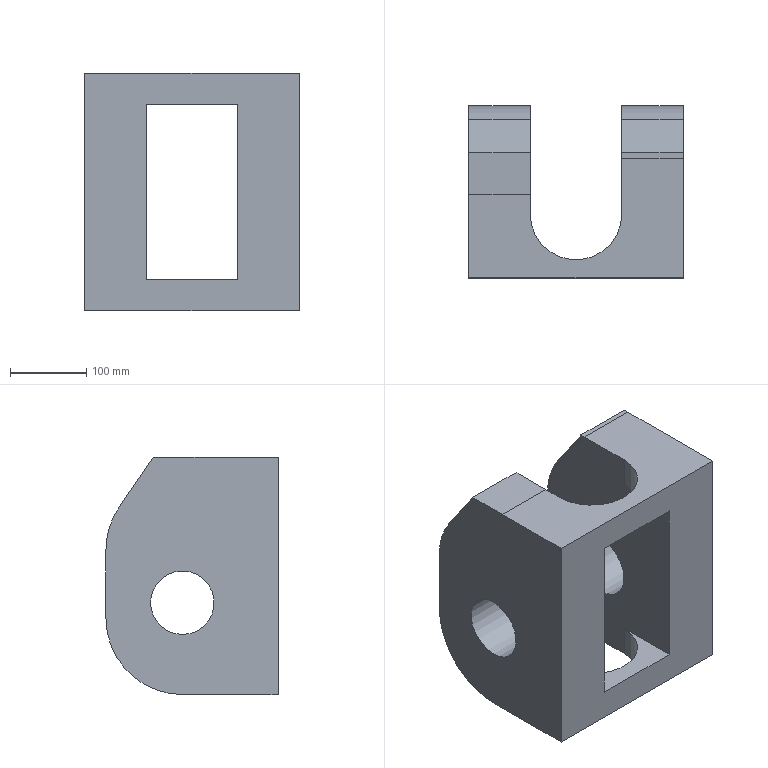Part | NX | features solid 2 | 1 solid | 25 faces | box 280 x 225 x 310 mm | volume 9841287 mm3 | plane 17 | cylinder 8 | commonest cylinder face diameters 200 x4 83 x2 120 x2
STEP:
#1=CARTESIAN_POINT('',(1335.,590.,10.));
#2=VERTEX_POINT('',#1);
#3=CARTESIAN_POINT('',(1215.,590.,10.));
#4=VERTEX_POINT('',#3);
#5=CARTESIAN_POINT('',(1495.,590.,10.));
#6=DIRECTION('',(-1.,0.,0.));
#7=VECTOR('',#6,1000.);
#8=LINE('',#5,#7);
#9=EDGE_CURVE('',#2,#4,#8,.T.);
#10=ORIENTED_EDGE('',*,*,#9,.T.);
#11=CARTESIAN_POINT('',(1215.,590.,240.));
#12=VERTEX_POINT('',#11);
#13=CARTESIAN_POINT('',(1215.,590.,-30.));
#14=DIRECTION('',(0.,0.,1.));
#15=VECTOR('',#14,1000.);
#16=LINE('',#13,#15);
#17=EDGE_CURVE('',#4,#12,#16,.T.);
#18=ORIENTED_EDGE('',*,*,#17,.T.);
#19=CARTESIAN_POINT('',(1335.,590.,240.));
#20=VERTEX_POINT('',#19);
#21=CARTESIAN_POINT('',(1440.,590.,240.));
#22=DIRECTION('',(-1.,0.,0.));
#23=VECTOR('',#22,1000.);
#24=LINE('',#21,#23);
#25=EDGE_CURVE('',#20,#12,#24,.T.);
#26=ORIENTED_EDGE('',*,*,#25,.F.);
#27=CARTESIAN_POINT('',(1335.,590.,-30.));
#28=DIRECTION('',(0.,0.,1.));
#29=VECTOR('',#28,1000.);
#30=LINE('',#27,#29);
#31=EDGE_CURVE('',#2,#20,#30,.T.);
#32=ORIENTED_EDGE('',*,*,#31,.F.);
#33=EDGE_LOOP('',(#10,#18,#26,#32));
#34=FACE_BOUND('',#33,.T.);
#35=CARTESIAN_POINT('',(1415.,590.,-30.));
#36=VERTEX_POINT('',#35);
#37=CARTESIAN_POINT('',(1415.,590.,280.));
#38=VERTEX_POINT('',#37);
#39=CARTESIAN_POINT('',(1415.,590.,-30.));
#40=DIRECTION('',(0.,0.,1.));
#41=VECTOR('',#40,1000.);
#42=LINE('',#39,#41);
#43=EDGE_CURVE('',#36,#38,#42,.T.);
#44=ORIENTED_EDGE('',*,*,#43,.T.);
#45=CARTESIAN_POINT('',(1135.,590.,280.));
#46=VERTEX_POINT('',#45);
#47=CARTESIAN_POINT('',(1405.,590.,280.));
#48=DIRECTION('',(-1.,0.,0.));
#49=VECTOR('',#48,1000.);
#50=LINE('',#47,#49);
#51=EDGE_CURVE('',#38,#46,#50,.T.);
#52=ORIENTED_EDGE('',*,*,#51,.T.);
#53=CARTESIAN_POINT('',(1135.,590.,-30.));
#54=VERTEX_POINT('',#53);
#55=CARTESIAN_POINT('',(1135.,590.,0.));
#56=DIRECTION('',(0.,0.,1.));
#57=VECTOR('',#56,1000.);
#58=LINE('',#55,#57);
#59=EDGE_CURVE('',#46,#54,#58,.F.);
#60=ORIENTED_EDGE('',*,*,#59,.T.);
#61=CARTESIAN_POINT('',(1135.,590.,-30.));
#62=DIRECTION('',(-1.,0.,0.));
#63=VECTOR('',#62,1000.);
#64=LINE('',#61,#63);
#65=EDGE_CURVE('',#36,#54,#64,.T.);
#66=ORIENTED_EDGE('',*,*,#65,.F.);
#67=EDGE_LOOP('',(#44,#52,#60,#66));
#68=FACE_BOUND('',#67,.T.);
#69=CARTESIAN_POINT('',(1135.,590.,0.));
#70=DIRECTION('',(0.,1.,0.));
#71=DIRECTION('',(0.,0.,-1.));
#72=AXIS2_PLACEMENT_3D('',#69,#70,#71);
#73=PLANE('',#72);
#74=ADVANCED_FACE('',(#34,#68),#73,.F.);
#75=ORIENTED_EDGE('',*,*,#51,.F.);
#76=CARTESIAN_POINT('',(1415.,746.5,280.));
#77=VERTEX_POINT('',#76);
#78=CARTESIAN_POINT('',(1415.,581.625,280.));
#79=DIRECTION('',(0.,-1.,0.));
#80=VECTOR('',#79,1000.);
#81=LINE('',#78,#80);
#82=EDGE_CURVE('',#38,#77,#81,.F.);
#83=ORIENTED_EDGE('',*,*,#82,.T.);
#84=CARTESIAN_POINT('',(1335.,746.5,280.));
#85=VERTEX_POINT('',#84);
#86=CARTESIAN_POINT('',(1405.,746.5,280.));
#87=DIRECTION('',(1.,0.,0.));
#88=VECTOR('',#87,1000.);
#89=LINE('',#86,#88);
#90=EDGE_CURVE('',#77,#85,#89,.F.);
#91=ORIENTED_EDGE('',*,*,#90,.T.);
#92=CARTESIAN_POINT('',(1335.,673.5,280.));
#93=VERTEX_POINT('',#92);
#94=CARTESIAN_POINT('',(1335.,590.,280.));
#95=DIRECTION('',(0.,-1.,0.));
#96=VECTOR('',#95,1000.);
#97=LINE('',#94,#96);
#98=EDGE_CURVE('',#93,#85,#97,.F.);
#99=ORIENTED_EDGE('',*,*,#98,.F.);
#100=CARTESIAN_POINT('',(1215.,673.5,280.));
#101=VERTEX_POINT('',#100);
#102=CARTESIAN_POINT('',(1275.,673.5,280.));
#103=DIRECTION('',(0.,0.,1.));
#104=DIRECTION('',(1.,0.,0.));
#105=AXIS2_PLACEMENT_3D('',#102,#103,#104);
#106=CIRCLE('',#105,60.);
#107=EDGE_CURVE('',#101,#93,#106,.T.);
#108=ORIENTED_EDGE('',*,*,#107,.F.);
#109=CARTESIAN_POINT('',(1215.,698.55,280.));
#110=VERTEX_POINT('',#109);
#111=CARTESIAN_POINT('',(1215.,581.625,280.));
#112=DIRECTION('',(0.,1.,0.));
#113=VECTOR('',#112,1000.);
#114=LINE('',#111,#113);
#115=EDGE_CURVE('',#110,#101,#114,.F.);
#116=ORIENTED_EDGE('',*,*,#115,.F.);
#117=CARTESIAN_POINT('',(1135.,698.55,280.));
#118=VERTEX_POINT('',#117);
#119=CARTESIAN_POINT('',(1405.,698.55,280.));
#120=DIRECTION('',(1.,0.,0.));
#121=VECTOR('',#120,1000.);
#122=LINE('',#119,#121);
#123=EDGE_CURVE('',#110,#118,#122,.F.);
#124=ORIENTED_EDGE('',*,*,#123,.T.);
#125=CARTESIAN_POINT('',(1135.,581.625,280.));
#126=DIRECTION('',(0.,-1.,0.));
#127=VECTOR('',#126,1000.);
#128=LINE('',#125,#127);
#129=EDGE_CURVE('',#46,#118,#128,.F.);
#130=ORIENTED_EDGE('',*,*,#129,.F.);
#131=EDGE_LOOP('',(#75,#83,#91,#99,#108,#116,#124,#130));
#132=FACE_BOUND('',#131,.T.);
#133=CARTESIAN_POINT('',(1405.,581.625,280.));
#134=DIRECTION('',(0.,0.,-1.));
#135=DIRECTION('',(-1.,0.,0.));
#136=AXIS2_PLACEMENT_3D('',#133,#134,#135);
#137=PLANE('',#136);
#138=ADVANCED_FACE('',(#132),#137,.F.);
#139=CARTESIAN_POINT('',(1135.,715.,-30.));
#140=VERTEX_POINT('',#139);
#141=CARTESIAN_POINT('',(1135.,530.,-30.));
#142=DIRECTION('',(0.,1.,0.));
#143=VECTOR('',#142,1000.);
#144=LINE('',#141,#143);
#145=EDGE_CURVE('',#140,#54,#144,.F.);
#146=ORIENTED_EDGE('',*,*,#145,.T.);
#147=ORIENTED_EDGE('',*,*,#59,.F.);
#148=ORIENTED_EDGE('',*,*,#129,.T.);
#149=CARTESIAN_POINT('',(1135.,753.35,280.));
#150=VERTEX_POINT('',#149);
#151=CARTESIAN_POINT('',(1135.,530.,280.));
#152=DIRECTION('',(0.,1.,0.));
#153=VECTOR('',#152,1000.);
#154=LINE('',#151,#153);
#155=EDGE_CURVE('',#150,#118,#154,.F.);
#156=ORIENTED_EDGE('',*,*,#155,.F.);
#157=CARTESIAN_POINT('',(1135.,797.5,215.547));
#158=VERTEX_POINT('',#157);
#159=CARTESIAN_POINT('',(1135.,826.551,173.137));
#160=DIRECTION('',(0.,-0.5651,0.825));
#161=VECTOR('',#160,1000.);
#162=LINE('',#159,#161);
#163=EDGE_CURVE('',#158,#150,#162,.T.);
#164=ORIENTED_EDGE('',*,*,#163,.F.);
#165=CARTESIAN_POINT('',(1135.,815.,159.034));
#166=VERTEX_POINT('',#165);
#167=CARTESIAN_POINT('',(1135.,715.,159.034));
#168=DIRECTION('',(-1.,0.,0.));
#169=DIRECTION('',(0.,0.,1.));
#170=AXIS2_PLACEMENT_3D('',#167,#168,#169);
#171=CIRCLE('',#170,100.);
#172=EDGE_CURVE('',#166,#158,#171,.F.);
#173=ORIENTED_EDGE('',*,*,#172,.F.);
#174=CARTESIAN_POINT('',(1135.,815.,70.));
#175=VERTEX_POINT('',#174);
#176=CARTESIAN_POINT('',(1135.,815.,-30.));
#177=DIRECTION('',(0.,0.,-1.));
#178=VECTOR('',#177,1000.);
#179=LINE('',#176,#178);
#180=EDGE_CURVE('',#175,#166,#179,.F.);
#181=ORIENTED_EDGE('',*,*,#180,.F.);
#182=CARTESIAN_POINT('',(1135.,715.,70.));
#183=DIRECTION('',(-1.,0.,0.));
#184=DIRECTION('',(0.,0.,1.));
#185=AXIS2_PLACEMENT_3D('',#182,#183,#184);
#186=CIRCLE('',#185,100.);
#187=EDGE_CURVE('',#140,#175,#186,.F.);
#188=ORIENTED_EDGE('',*,*,#187,.F.);
#189=EDGE_LOOP('',(#146,#147,#148,#156,#164,#173,#181,#188));
#190=FACE_BOUND('',#189,.T.);
#191=CARTESIAN_POINT('',(1135.,715.,48.5));
#192=VERTEX_POINT('',#191);
#193=CARTESIAN_POINT('',(1135.,715.,90.));
#194=DIRECTION('',(1.,0.,0.));
#195=DIRECTION('',(0.,0.,-1.));
#196=AXIS2_PLACEMENT_3D('',#193,#194,#195);
#197=CIRCLE('',#196,41.5);
#198=EDGE_CURVE('',#192,#192,#197,.T.);
#199=ORIENTED_EDGE('',*,*,#198,.T.);
#200=EDGE_LOOP('',(#199));
#201=FACE_BOUND('',#200,.T.);
#202=CARTESIAN_POINT('',(1135.,530.,-30.));
#203=DIRECTION('',(1.,0.,0.));
#204=DIRECTION('',(0.,0.,-1.));
#205=AXIS2_PLACEMENT_3D('',#202,#203,#204);
#206=PLANE('',#205);
#207=ADVANCED_FACE('',(#190,#201),#206,.F.);
#208=CARTESIAN_POINT('',(1335.,715.,48.5));
#209=VERTEX_POINT('',#208);
#210=CARTESIAN_POINT('',(1335.,715.,90.));
#211=DIRECTION('',(1.,0.,0.));
#212=DIRECTION('',(0.,0.,-1.));
#213=AXIS2_PLACEMENT_3D('',#210,#211,#212);
#214=CIRCLE('',#213,41.5);
#215=EDGE_CURVE('',#209,#209,#214,.T.);
#216=ORIENTED_EDGE('',*,*,#215,.T.);
#217=EDGE_LOOP('',(#216));
#218=FACE_BOUND('',#217,.T.);
#219=CARTESIAN_POINT('',(1335.,749.714,280.));
#220=VERTEX_POINT('',#219);
#221=CARTESIAN_POINT('',(1335.,590.,280.));
#222=DIRECTION('',(0.,1.,0.));
#223=VECTOR('',#222,1000.);
#224=LINE('',#221,#223);
#225=EDGE_CURVE('',#220,#85,#224,.F.);
#226=ORIENTED_EDGE('',*,*,#225,.F.);
#227=CARTESIAN_POINT('',(1335.,795.025,213.852));
#228=VERTEX_POINT('',#227);
#229=CARTESIAN_POINT('',(1335.,795.025,213.852));
#230=DIRECTION('',(0.,-0.5651,0.825));
#231=VECTOR('',#230,1000.);
#232=LINE('',#229,#231);
#233=EDGE_CURVE('',#220,#228,#232,.F.);
#234=ORIENTED_EDGE('',*,*,#233,.T.);
#235=CARTESIAN_POINT('',(1335.,812.,159.034));
#236=VERTEX_POINT('',#235);
#237=CARTESIAN_POINT('',(1335.,715.,159.034));
#238=DIRECTION('',(1.,0.,0.));
#239=DIRECTION('',(0.,0.,-1.));
#240=AXIS2_PLACEMENT_3D('',#237,#238,#239);
#241=CIRCLE('',#240,97.);
#242=EDGE_CURVE('',#228,#236,#241,.F.);
#243=ORIENTED_EDGE('',*,*,#242,.T.);
#244=CARTESIAN_POINT('',(1335.,812.,70.));
#245=VERTEX_POINT('',#244);
#246=CARTESIAN_POINT('',(1335.,812.,70.));
#247=DIRECTION('',(0.,0.,1.));
#248=VECTOR('',#247,1000.);
#249=LINE('',#246,#248);
#250=EDGE_CURVE('',#236,#245,#249,.F.);
#251=ORIENTED_EDGE('',*,*,#250,.T.);
#252=CARTESIAN_POINT('',(1335.,715.,-27.));
#253=VERTEX_POINT('',#252);
#254=CARTESIAN_POINT('',(1335.,715.,70.));
#255=DIRECTION('',(1.,0.,0.));
#256=DIRECTION('',(0.,0.,-1.));
#257=AXIS2_PLACEMENT_3D('',#254,#255,#256);
#258=CIRCLE('',#257,97.);
#259=EDGE_CURVE('',#245,#253,#258,.F.);
#260=ORIENTED_EDGE('',*,*,#259,.T.);
#261=CARTESIAN_POINT('',(1335.,673.5,-27.));
#262=VERTEX_POINT('',#261);
#263=CARTESIAN_POINT('',(1335.,673.5,-27.));
#264=DIRECTION('',(0.,1.,0.));
#265=VECTOR('',#264,1000.);
#266=LINE('',#263,#265);
#267=EDGE_CURVE('',#253,#262,#266,.F.);
#268=ORIENTED_EDGE('',*,*,#267,.T.);
#269=CARTESIAN_POINT('',(1335.,673.5,10.));
#270=VERTEX_POINT('',#269);
#271=CARTESIAN_POINT('',(1335.,673.5,-30.));
#272=DIRECTION('',(0.,0.,1.));
#273=VECTOR('',#272,1000.);
#274=LINE('',#271,#273);
#275=EDGE_CURVE('',#262,#270,#274,.T.);
#276=ORIENTED_EDGE('',*,*,#275,.T.);
#277=CARTESIAN_POINT('',(1335.,590.,10.));
#278=DIRECTION('',(0.,1.,0.));
#279=VECTOR('',#278,1000.);
#280=LINE('',#277,#279);
#281=EDGE_CURVE('',#2,#270,#280,.T.);
#282=ORIENTED_EDGE('',*,*,#281,.F.);
#283=ORIENTED_EDGE('',*,*,#31,.T.);
#284=CARTESIAN_POINT('',(1335.,673.5,240.));
#285=VERTEX_POINT('',#284);
#286=CARTESIAN_POINT('',(1335.,690.,240.));
#287=DIRECTION('',(0.,1.,0.));
#288=VECTOR('',#287,1000.);
#289=LINE('',#286,#288);
#290=EDGE_CURVE('',#20,#285,#289,.T.);
#291=ORIENTED_EDGE('',*,*,#290,.T.);
#292=CARTESIAN_POINT('',(1335.,673.5,330.));
#293=DIRECTION('',(0.,0.,-1.));
#294=VECTOR('',#293,1000.);
#295=LINE('',#292,#294);
#296=EDGE_CURVE('',#93,#285,#295,.T.);
#297=ORIENTED_EDGE('',*,*,#296,.F.);
#298=ORIENTED_EDGE('',*,*,#98,.T.);
#299=EDGE_LOOP('',(#226,#234,#243,#251,#260,#268,#276,#282,#283,#291,#297,#298));
#300=FACE_BOUND('',#299,.T.);
#301=CARTESIAN_POINT('',(1335.,590.,-30.));
#302=DIRECTION('',(1.,0.,0.));
#303=DIRECTION('',(0.,0.,-1.));
#304=AXIS2_PLACEMENT_3D('',#301,#302,#303);
#305=PLANE('',#304);
#306=ADVANCED_FACE('',(#218,#300),#305,.F.);
#307=CARTESIAN_POINT('',(1215.,715.,48.5));
#308=VERTEX_POINT('',#307);
#309=CARTESIAN_POINT('',(1215.,715.,90.));
#310=DIRECTION('',(1.,0.,0.));
#311=DIRECTION('',(0.,0.,-1.));
#312=AXIS2_PLACEMENT_3D('',#309,#310,#311);
#313=CIRCLE('',#312,41.5);
#314=EDGE_CURVE('',#308,#308,#313,.T.);
#315=ORIENTED_EDGE('',*,*,#314,.F.);
#316=EDGE_LOOP('',(#315));
#317=FACE_BOUND('',#316,.T.);
#318=CARTESIAN_POINT('',(1215.,795.025,213.852));
#319=VERTEX_POINT('',#318);
#320=CARTESIAN_POINT('',(1215.,749.714,280.));
#321=VERTEX_POINT('',#320);
#322=CARTESIAN_POINT('',(1215.,843.238,143.468));
#323=DIRECTION('',(0.,0.5651,-0.825));
#324=VECTOR('',#323,1000.);
#325=LINE('',#322,#324);
#326=EDGE_CURVE('',#319,#321,#325,.F.);
#327=ORIENTED_EDGE('',*,*,#326,.T.);
#328=CARTESIAN_POINT('',(1215.,590.,280.));
#329=DIRECTION('',(0.,1.,0.));
#330=VECTOR('',#329,1000.);
#331=LINE('',#328,#330);
#332=EDGE_CURVE('',#321,#110,#331,.F.);
#333=ORIENTED_EDGE('',*,*,#332,.T.);
#334=ORIENTED_EDGE('',*,*,#115,.T.);
#335=CARTESIAN_POINT('',(1215.,673.5,240.));
#336=VERTEX_POINT('',#335);
#337=CARTESIAN_POINT('',(1215.,673.5,330.));
#338=DIRECTION('',(0.,0.,-1.));
#339=VECTOR('',#338,1000.);
#340=LINE('',#337,#339);
#341=EDGE_CURVE('',#101,#336,#340,.T.);
#342=ORIENTED_EDGE('',*,*,#341,.T.);
#343=CARTESIAN_POINT('',(1215.,690.,240.));
#344=DIRECTION('',(0.,1.,0.));
#345=VECTOR('',#344,1000.);
#346=LINE('',#343,#345);
#347=EDGE_CURVE('',#12,#336,#346,.T.);
#348=ORIENTED_EDGE('',*,*,#347,.F.);
#349=ORIENTED_EDGE('',*,*,#17,.F.);
#350=CARTESIAN_POINT('',(1215.,673.5,10.));
#351=VERTEX_POINT('',#350);
#352=CARTESIAN_POINT('',(1215.,590.,10.));
#353=DIRECTION('',(0.,1.,0.));
#354=VECTOR('',#353,1000.);
#355=LINE('',#352,#354);
#356=EDGE_CURVE('',#4,#351,#355,.T.);
#357=ORIENTED_EDGE('',*,*,#356,.T.);
#358=CARTESIAN_POINT('',(1215.,673.5,-27.));
#359=VERTEX_POINT('',#358);
#360=CARTESIAN_POINT('',(1215.,673.5,-30.));
#361=DIRECTION('',(0.,0.,1.));
#362=VECTOR('',#361,1000.);
#363=LINE('',#360,#362);
#364=EDGE_CURVE('',#359,#351,#363,.T.);
#365=ORIENTED_EDGE('',*,*,#364,.F.);
#366=CARTESIAN_POINT('',(1215.,715.,-27.));
#367=VERTEX_POINT('',#366);
#368=CARTESIAN_POINT('',(1215.,590.,-27.));
#369=DIRECTION('',(0.,1.,0.));
#370=VECTOR('',#369,1000.);
#371=LINE('',#368,#370);
#372=EDGE_CURVE('',#359,#367,#371,.T.);
#373=ORIENTED_EDGE('',*,*,#372,.T.);
#374=CARTESIAN_POINT('',(1215.,812.,70.));
#375=VERTEX_POINT('',#374);
#376=CARTESIAN_POINT('',(1215.,715.,70.));
#377=DIRECTION('',(1.,0.,0.));
#378=DIRECTION('',(0.,0.,-1.));
#379=AXIS2_PLACEMENT_3D('',#376,#377,#378);
#380=CIRCLE('',#379,97.);
#381=EDGE_CURVE('',#367,#375,#380,.T.);
#382=ORIENTED_EDGE('',*,*,#381,.T.);
#383=CARTESIAN_POINT('',(1215.,812.,159.034));
#384=VERTEX_POINT('',#383);
#385=CARTESIAN_POINT('',(1215.,812.,-30.));
#386=DIRECTION('',(0.,0.,1.));
#387=VECTOR('',#386,1000.);
#388=LINE('',#385,#387);
#389=EDGE_CURVE('',#375,#384,#388,.T.);
#390=ORIENTED_EDGE('',*,*,#389,.T.);
#391=CARTESIAN_POINT('',(1215.,715.,159.034));
#392=DIRECTION('',(1.,0.,0.));
#393=DIRECTION('',(0.,0.,-1.));
#394=AXIS2_PLACEMENT_3D('',#391,#392,#393);
#395=CIRCLE('',#394,97.);
#396=EDGE_CURVE('',#384,#319,#395,.T.);
#397=ORIENTED_EDGE('',*,*,#396,.T.);
#398=EDGE_LOOP('',(#327,#333,#334,#342,#348,#349,#357,#365,#373,#382,#390,#397));
#399=FACE_BOUND('',#398,.T.);
#400=CARTESIAN_POINT('',(1215.,590.,-30.));
#401=DIRECTION('',(1.,0.,0.));
#402=DIRECTION('',(0.,0.,-1.));
#403=AXIS2_PLACEMENT_3D('',#400,#401,#402);
#404=PLANE('',#403);
#405=ADVANCED_FACE('',(#317,#399),#404,.T.);
#406=ORIENTED_EDGE('',*,*,#82,.F.);
#407=ORIENTED_EDGE('',*,*,#43,.F.);
#408=CARTESIAN_POINT('',(1415.,715.,-30.));
#409=VERTEX_POINT('',#408);
#410=CARTESIAN_POINT('',(1415.,530.,-30.));
#411=DIRECTION('',(0.,1.,0.));
#412=VECTOR('',#411,1000.);
#413=LINE('',#410,#412);
#414=EDGE_CURVE('',#36,#409,#413,.T.);
#415=ORIENTED_EDGE('',*,*,#414,.T.);
#416=CARTESIAN_POINT('',(1415.,815.,70.));
#417=VERTEX_POINT('',#416);
#418=CARTESIAN_POINT('',(1415.,715.,70.));
#419=DIRECTION('',(-1.,0.,0.));
#420=DIRECTION('',(0.,0.,1.));
#421=AXIS2_PLACEMENT_3D('',#418,#419,#420);
#422=CIRCLE('',#421,100.);
#423=EDGE_CURVE('',#417,#409,#422,.T.);
#424=ORIENTED_EDGE('',*,*,#423,.F.);
#425=CARTESIAN_POINT('',(1415.,815.,159.034));
#426=VERTEX_POINT('',#425);
#427=CARTESIAN_POINT('',(1415.,815.,-30.));
#428=DIRECTION('',(0.,0.,1.));
#429=VECTOR('',#428,1000.);
#430=LINE('',#427,#429);
#431=EDGE_CURVE('',#426,#417,#430,.F.);
#432=ORIENTED_EDGE('',*,*,#431,.F.);
#433=CARTESIAN_POINT('',(1415.,797.5,215.547));
#434=VERTEX_POINT('',#433);
#435=CARTESIAN_POINT('',(1415.,715.,159.034));
#436=DIRECTION('',(-1.,0.,0.));
#437=DIRECTION('',(0.,0.,1.));
#438=AXIS2_PLACEMENT_3D('',#435,#436,#437);
#439=CIRCLE('',#438,100.);
#440=EDGE_CURVE('',#434,#426,#439,.T.);
#441=ORIENTED_EDGE('',*,*,#440,.F.);
#442=CARTESIAN_POINT('',(1415.,753.35,280.));
#443=VERTEX_POINT('',#442);
#444=CARTESIAN_POINT('',(1415.,845.713,145.163));
#445=DIRECTION('',(0.,-0.5651,0.825));
#446=VECTOR('',#445,1000.);
#447=LINE('',#444,#446);
#448=EDGE_CURVE('',#443,#434,#447,.F.);
#449=ORIENTED_EDGE('',*,*,#448,.F.);
#450=CARTESIAN_POINT('',(1415.,530.,280.));
#451=DIRECTION('',(0.,1.,0.));
#452=VECTOR('',#451,1000.);
#453=LINE('',#450,#452);
#454=EDGE_CURVE('',#443,#77,#453,.F.);
#455=ORIENTED_EDGE('',*,*,#454,.T.);
#456=EDGE_LOOP('',(#406,#407,#415,#424,#432,#441,#449,#455));
#457=FACE_BOUND('',#456,.T.);
#458=CARTESIAN_POINT('',(1415.,715.,131.5));
#459=VERTEX_POINT('',#458);
#460=CARTESIAN_POINT('',(1415.,715.,90.));
#461=DIRECTION('',(-1.,0.,0.));
#462=DIRECTION('',(0.,0.,1.));
#463=AXIS2_PLACEMENT_3D('',#460,#461,#462);
#464=CIRCLE('',#463,41.5);
#465=EDGE_CURVE('',#459,#459,#464,.T.);
#466=ORIENTED_EDGE('',*,*,#465,.T.);
#467=EDGE_LOOP('',(#466));
#468=FACE_BOUND('',#467,.T.);
#469=CARTESIAN_POINT('',(1415.,530.,-30.));
#470=DIRECTION('',(1.,0.,0.));
#471=DIRECTION('',(0.,0.,-1.));
#472=AXIS2_PLACEMENT_3D('',#469,#470,#471);
#473=PLANE('',#472);
#474=ADVANCED_FACE('',(#457,#468),#473,.T.);
#475=ORIENTED_EDGE('',*,*,#107,.T.);
#476=ORIENTED_EDGE('',*,*,#296,.T.);
#477=CARTESIAN_POINT('',(1275.,673.5,240.));
#478=DIRECTION('',(0.,0.,1.));
#479=DIRECTION('',(1.,0.,0.));
#480=AXIS2_PLACEMENT_3D('',#477,#478,#479);
#481=CIRCLE('',#480,60.);
#482=EDGE_CURVE('',#285,#336,#481,.F.);
#483=ORIENTED_EDGE('',*,*,#482,.T.);
#484=ORIENTED_EDGE('',*,*,#341,.F.);
#485=EDGE_LOOP('',(#475,#476,#483,#484));
#486=FACE_BOUND('',#485,.T.);
#487=CARTESIAN_POINT('',(1275.,673.5,330.));
#488=DIRECTION('',(0.,0.,-1.));
#489=DIRECTION('',(-1.,0.,0.));
#490=AXIS2_PLACEMENT_3D('',#487,#488,#489);
#491=CYLINDRICAL_SURFACE('',#490,60.);
#492=ADVANCED_FACE('',(#486),#491,.F.);
#493=ORIENTED_EDGE('',*,*,#233,.F.);
#494=CARTESIAN_POINT('',(1335.,753.35,280.));
#495=VERTEX_POINT('',#494);
#496=CARTESIAN_POINT('',(1335.,581.625,280.));
#497=DIRECTION('',(0.,-1.,0.));
#498=VECTOR('',#497,1000.);
#499=LINE('',#496,#498);
#500=EDGE_CURVE('',#495,#220,#499,.T.);
#501=ORIENTED_EDGE('',*,*,#500,.F.);
#502=CARTESIAN_POINT('',(1335.,797.5,215.547));
#503=VERTEX_POINT('',#502);
#504=CARTESIAN_POINT('',(1335.,845.713,145.163));
#505=DIRECTION('',(0.,-0.5651,0.825));
#506=VECTOR('',#505,1000.);
#507=LINE('',#504,#506);
#508=EDGE_CURVE('',#503,#495,#507,.T.);
#509=ORIENTED_EDGE('',*,*,#508,.F.);
#510=CARTESIAN_POINT('',(1335.,815.,159.034));
#511=VERTEX_POINT('',#510);
#512=CARTESIAN_POINT('',(1335.,715.,159.034));
#513=DIRECTION('',(-1.,0.,0.));
#514=DIRECTION('',(0.,0.,1.));
#515=AXIS2_PLACEMENT_3D('',#512,#513,#514);
#516=CIRCLE('',#515,100.);
#517=EDGE_CURVE('',#511,#503,#516,.F.);
#518=ORIENTED_EDGE('',*,*,#517,.F.);
#519=CARTESIAN_POINT('',(1335.,815.,70.));
#520=VERTEX_POINT('',#519);
#521=CARTESIAN_POINT('',(1335.,815.,-30.));
#522=DIRECTION('',(0.,0.,-1.));
#523=VECTOR('',#522,1000.);
#524=LINE('',#521,#523);
#525=EDGE_CURVE('',#520,#511,#524,.F.);
#526=ORIENTED_EDGE('',*,*,#525,.F.);
#527=CARTESIAN_POINT('',(1335.,715.,-30.));
#528=VERTEX_POINT('',#527);
#529=CARTESIAN_POINT('',(1335.,715.,70.));
#530=DIRECTION('',(-1.,0.,0.));
#531=DIRECTION('',(0.,0.,1.));
#532=AXIS2_PLACEMENT_3D('',#529,#530,#531);
#533=CIRCLE('',#532,100.);
#534=EDGE_CURVE('',#528,#520,#533,.F.);
#535=ORIENTED_EDGE('',*,*,#534,.F.);
#536=CARTESIAN_POINT('',(1335.,673.5,-30.));
#537=VERTEX_POINT('',#536);
#538=CARTESIAN_POINT('',(1335.,590.,-30.));
#539=DIRECTION('',(0.,-1.,0.));
#540=VECTOR('',#539,1000.);
#541=LINE('',#538,#540);
#542=EDGE_CURVE('',#537,#528,#541,.F.);
#543=ORIENTED_EDGE('',*,*,#542,.F.);
#544=CARTESIAN_POINT('',(1335.,673.5,-30.));
#545=DIRECTION('',(0.,0.,1.));
#546=VECTOR('',#545,1000.);
#547=LINE('',#544,#546);
#548=EDGE_CURVE('',#262,#537,#547,.F.);
#549=ORIENTED_EDGE('',*,*,#548,.F.);
#550=ORIENTED_EDGE('',*,*,#267,.F.);
#551=ORIENTED_EDGE('',*,*,#259,.F.);
#552=ORIENTED_EDGE('',*,*,#250,.F.);
#553=ORIENTED_EDGE('',*,*,#242,.F.);
#554=EDGE_LOOP('',(#493,#501,#509,#518,#526,#535,#543,#549,#550,#551,#552,#553));
#555=FACE_BOUND('',#554,.T.);
#556=CARTESIAN_POINT('',(1335.,590.,-30.));
#557=DIRECTION('',(1.,0.,0.));
#558=DIRECTION('',(0.,0.,-1.));
#559=AXIS2_PLACEMENT_3D('',#556,#557,#558);
#560=PLANE('',#559);
#561=ADVANCED_FACE('',(#555),#560,.F.);
#562=ORIENTED_EDGE('',*,*,#65,.T.);
#563=ORIENTED_EDGE('',*,*,#145,.F.);
#564=CARTESIAN_POINT('',(1215.,715.,-30.));
#565=VERTEX_POINT('',#564);
#566=CARTESIAN_POINT('',(1405.,715.,-30.));
#567=DIRECTION('',(-1.,0.,0.));
#568=VECTOR('',#567,1000.);
#569=LINE('',#566,#568);
#570=EDGE_CURVE('',#140,#565,#569,.F.);
#571=ORIENTED_EDGE('',*,*,#570,.T.);
#572=CARTESIAN_POINT('',(1215.,673.5,-30.));
#573=VERTEX_POINT('',#572);
#574=CARTESIAN_POINT('',(1215.,590.,-30.));
#575=DIRECTION('',(0.,-1.,0.));
#576=VECTOR('',#575,1000.);
#577=LINE('',#574,#576);
#578=EDGE_CURVE('',#565,#573,#577,.T.);
#579=ORIENTED_EDGE('',*,*,#578,.T.);
#580=CARTESIAN_POINT('',(1275.,673.5,-30.));
#581=DIRECTION('',(0.,0.,1.));
#582=DIRECTION('',(1.,0.,0.));
#583=AXIS2_PLACEMENT_3D('',#580,#581,#582);
#584=CIRCLE('',#583,60.);
#585=EDGE_CURVE('',#573,#537,#584,.T.);
#586=ORIENTED_EDGE('',*,*,#585,.T.);
#587=ORIENTED_EDGE('',*,*,#542,.T.);
#588=CARTESIAN_POINT('',(1405.,715.,-30.));
#589=DIRECTION('',(-1.,0.,0.));
#590=VECTOR('',#589,1000.);
#591=LINE('',#588,#590);
#592=EDGE_CURVE('',#528,#409,#591,.F.);
#593=ORIENTED_EDGE('',*,*,#592,.T.);
#594=ORIENTED_EDGE('',*,*,#414,.F.);
#595=EDGE_LOOP('',(#562,#563,#571,#579,#586,#587,#593,#594));
#596=FACE_BOUND('',#595,.T.);
#597=CARTESIAN_POINT('',(1405.,581.625,-30.));
#598=DIRECTION('',(0.,0.,-1.));
#599=DIRECTION('',(-1.,0.,0.));
#600=AXIS2_PLACEMENT_3D('',#597,#598,#599);
#601=PLANE('',#600);
#602=ADVANCED_FACE('',(#596),#601,.T.);
#603=CARTESIAN_POINT('',(1415.,815.,70.));
#604=DIRECTION('',(-1.,0.,0.));
#605=VECTOR('',#604,1000.);
#606=LINE('',#603,#605);
#607=EDGE_CURVE('',#417,#520,#606,.T.);
#608=ORIENTED_EDGE('',*,*,#607,.T.);
#609=ORIENTED_EDGE('',*,*,#525,.T.);
#610=CARTESIAN_POINT('',(1415.,815.,159.034));
#611=DIRECTION('',(-1.,0.,0.));
#612=VECTOR('',#611,1000.);
#613=LINE('',#610,#612);
#614=EDGE_CURVE('',#511,#426,#613,.F.);
#615=ORIENTED_EDGE('',*,*,#614,.T.);
#616=ORIENTED_EDGE('',*,*,#431,.T.);
#617=EDGE_LOOP('',(#608,#609,#615,#616));
#618=FACE_BOUND('',#617,.T.);
#619=CARTESIAN_POINT('',(1415.,815.,-30.));
#620=DIRECTION('',(0.,1.,0.));
#621=DIRECTION('',(0.,0.,-1.));
#622=AXIS2_PLACEMENT_3D('',#619,#620,#621);
#623=PLANE('',#622);
#624=ADVANCED_FACE('',(#618),#623,.T.);
#625=CARTESIAN_POINT('',(1215.,815.,70.));
#626=VERTEX_POINT('',#625);
#627=CARTESIAN_POINT('',(1215.,815.,70.));
#628=DIRECTION('',(-1.,0.,0.));
#629=VECTOR('',#628,1000.);
#630=LINE('',#627,#629);
#631=EDGE_CURVE('',#626,#175,#630,.T.);
#632=ORIENTED_EDGE('',*,*,#631,.T.);
#633=ORIENTED_EDGE('',*,*,#180,.T.);
#634=CARTESIAN_POINT('',(1215.,815.,159.034));
#635=VERTEX_POINT('',#634);
#636=CARTESIAN_POINT('',(1215.,815.,159.034));
#637=DIRECTION('',(-1.,0.,0.));
#638=VECTOR('',#637,1000.);
#639=LINE('',#636,#638);
#640=EDGE_CURVE('',#166,#635,#639,.F.);
#641=ORIENTED_EDGE('',*,*,#640,.T.);
#642=CARTESIAN_POINT('',(1215.,815.,-30.));
#643=DIRECTION('',(0.,0.,-1.));
#644=VECTOR('',#643,1000.);
#645=LINE('',#642,#644);
#646=EDGE_CURVE('',#635,#626,#645,.T.);
#647=ORIENTED_EDGE('',*,*,#646,.T.);
#648=EDGE_LOOP('',(#632,#633,#641,#647));
#649=FACE_BOUND('',#648,.T.);
#650=CARTESIAN_POINT('',(1215.,815.,-30.));
#651=DIRECTION('',(0.,1.,0.));
#652=DIRECTION('',(0.,0.,-1.));
#653=AXIS2_PLACEMENT_3D('',#650,#651,#652);
#654=PLANE('',#653);
#655=ADVANCED_FACE('',(#649),#654,.T.);
#656=ORIENTED_EDGE('',*,*,#364,.T.);
#657=CARTESIAN_POINT('',(1275.,673.5,10.));
#658=DIRECTION('',(0.,0.,-1.));
#659=DIRECTION('',(-1.,0.,0.));
#660=AXIS2_PLACEMENT_3D('',#657,#658,#659);
#661=CIRCLE('',#660,60.);
#662=EDGE_CURVE('',#351,#270,#661,.F.);
#663=ORIENTED_EDGE('',*,*,#662,.T.);
#664=ORIENTED_EDGE('',*,*,#275,.F.);
#665=ORIENTED_EDGE('',*,*,#548,.T.);
#666=ORIENTED_EDGE('',*,*,#585,.F.);
#667=CARTESIAN_POINT('',(1215.,673.5,-30.));
#668=DIRECTION('',(0.,0.,1.));
#669=VECTOR('',#668,1000.);
#670=LINE('',#667,#669);
#671=EDGE_CURVE('',#359,#573,#670,.F.);
#672=ORIENTED_EDGE('',*,*,#671,.F.);
#673=EDGE_LOOP('',(#656,#663,#664,#665,#666,#672));
#674=FACE_BOUND('',#673,.T.);
#675=CARTESIAN_POINT('',(1275.,673.5,-30.));
#676=DIRECTION('',(0.,0.,1.));
#677=DIRECTION('',(1.,0.,0.));
#678=AXIS2_PLACEMENT_3D('',#675,#676,#677);
#679=CYLINDRICAL_SURFACE('',#678,60.);
#680=ADVANCED_FACE('',(#674),#679,.F.);
#681=ORIENTED_EDGE('',*,*,#281,.T.);
#682=ORIENTED_EDGE('',*,*,#662,.F.);
#683=ORIENTED_EDGE('',*,*,#356,.F.);
#684=ORIENTED_EDGE('',*,*,#9,.F.);
#685=EDGE_LOOP('',(#681,#682,#683,#684));
#686=FACE_BOUND('',#685,.T.);
#687=CARTESIAN_POINT('',(1285.,659.625,10.));
#688=DIRECTION('',(0.,0.,1.));
#689=DIRECTION('',(1.,0.,0.));
#690=AXIS2_PLACEMENT_3D('',#687,#688,#689);
#691=PLANE('',#690);
#692=ADVANCED_FACE('',(#686),#691,.T.);
#693=ORIENTED_EDGE('',*,*,#570,.F.);
#694=ORIENTED_EDGE('',*,*,#187,.T.);
#695=ORIENTED_EDGE('',*,*,#631,.F.);
#696=CARTESIAN_POINT('',(1215.,715.,70.));
#697=DIRECTION('',(-1.,0.,0.));
#698=DIRECTION('',(0.,0.,1.));
#699=AXIS2_PLACEMENT_3D('',#696,#697,#698);
#700=CIRCLE('',#699,100.);
#701=EDGE_CURVE('',#626,#565,#700,.T.);
#702=ORIENTED_EDGE('',*,*,#701,.T.);
#703=EDGE_LOOP('',(#693,#694,#695,#702));
#704=FACE_BOUND('',#703,.T.);
#705=CARTESIAN_POINT('',(1215.,715.,70.));
#706=DIRECTION('',(-1.,0.,0.));
#707=DIRECTION('',(0.,0.,1.));
#708=AXIS2_PLACEMENT_3D('',#705,#706,#707);
#709=CYLINDRICAL_SURFACE('',#708,100.);
#710=ADVANCED_FACE('',(#704),#709,.T.);
#711=ORIENTED_EDGE('',*,*,#592,.F.);
#712=ORIENTED_EDGE('',*,*,#534,.T.);
#713=ORIENTED_EDGE('',*,*,#607,.F.);
#714=ORIENTED_EDGE('',*,*,#423,.T.);
#715=EDGE_LOOP('',(#711,#712,#713,#714));
#716=FACE_BOUND('',#715,.T.);
#717=CARTESIAN_POINT('',(1415.,715.,70.));
#718=DIRECTION('',(-1.,0.,0.));
#719=DIRECTION('',(0.,0.,1.));
#720=AXIS2_PLACEMENT_3D('',#717,#718,#719);
#721=CYLINDRICAL_SURFACE('',#720,100.);
#722=ADVANCED_FACE('',(#716),#721,.T.);
#723=ORIENTED_EDGE('',*,*,#465,.F.);
#724=EDGE_LOOP('',(#723));
#725=FACE_BOUND('',#724,.T.);
#726=ORIENTED_EDGE('',*,*,#215,.F.);
#727=EDGE_LOOP('',(#726));
#728=FACE_BOUND('',#727,.T.);
#729=CARTESIAN_POINT('',(1415.,715.,90.));
#730=DIRECTION('',(-1.,0.,0.));
#731=DIRECTION('',(0.,0.,1.));
#732=AXIS2_PLACEMENT_3D('',#729,#730,#731);
#733=CYLINDRICAL_SURFACE('',#732,41.5);
#734=ADVANCED_FACE('',(#725,#728),#733,.F.);
#735=ORIENTED_EDGE('',*,*,#314,.T.);
#736=EDGE_LOOP('',(#735));
#737=FACE_BOUND('',#736,.T.);
#738=ORIENTED_EDGE('',*,*,#198,.F.);
#739=EDGE_LOOP('',(#738));
#740=FACE_BOUND('',#739,.T.);
#741=CARTESIAN_POINT('',(1415.,715.,90.));
#742=DIRECTION('',(-1.,0.,0.));
#743=DIRECTION('',(0.,0.,1.));
#744=AXIS2_PLACEMENT_3D('',#741,#742,#743);
#745=CYLINDRICAL_SURFACE('',#744,41.5);
#746=ADVANCED_FACE('',(#737,#740),#745,.F.);
#747=CARTESIAN_POINT('',(1360.,797.5,215.547));
#748=DIRECTION('',(1.,0.,0.));
#749=VECTOR('',#748,1000.);
#750=LINE('',#747,#749);
#751=EDGE_CURVE('',#434,#503,#750,.F.);
#752=ORIENTED_EDGE('',*,*,#751,.T.);
#753=ORIENTED_EDGE('',*,*,#508,.T.);
#754=CARTESIAN_POINT('',(1405.,753.35,280.));
#755=DIRECTION('',(-1.,0.,0.));
#756=VECTOR('',#755,1000.);
#757=LINE('',#754,#756);
#758=EDGE_CURVE('',#443,#495,#757,.T.);
#759=ORIENTED_EDGE('',*,*,#758,.F.);
#760=ORIENTED_EDGE('',*,*,#448,.T.);
#761=EDGE_LOOP('',(#752,#753,#759,#760));
#762=FACE_BOUND('',#761,.T.);
#763=CARTESIAN_POINT('',(1360.,746.5,290.));
#764=DIRECTION('',(0.,-0.825,-0.5651));
#765=DIRECTION('',(0.,-0.5651,0.825));
#766=AXIS2_PLACEMENT_3D('',#763,#764,#765);
#767=PLANE('',#766);
#768=ADVANCED_FACE('',(#762),#767,.F.);
#769=CARTESIAN_POINT('',(1215.,753.35,280.));
#770=VERTEX_POINT('',#769);
#771=CARTESIAN_POINT('',(1210.,753.35,280.));
#772=DIRECTION('',(1.,0.,0.));
#773=VECTOR('',#772,1000.);
#774=LINE('',#771,#773);
#775=EDGE_CURVE('',#770,#150,#774,.F.);
#776=ORIENTED_EDGE('',*,*,#775,.F.);
#777=CARTESIAN_POINT('',(1215.,797.5,215.547));
#778=VERTEX_POINT('',#777);
#779=CARTESIAN_POINT('',(1215.,845.713,145.163));
#780=DIRECTION('',(0.,-0.5651,0.825));
#781=VECTOR('',#780,1000.);
#782=LINE('',#779,#781);
#783=EDGE_CURVE('',#770,#778,#782,.F.);
#784=ORIENTED_EDGE('',*,*,#783,.T.);
#785=CARTESIAN_POINT('',(1210.,797.5,215.547));
#786=DIRECTION('',(1.,0.,0.));
#787=VECTOR('',#786,1000.);
#788=LINE('',#785,#787);
#789=EDGE_CURVE('',#778,#158,#788,.F.);
#790=ORIENTED_EDGE('',*,*,#789,.T.);
#791=ORIENTED_EDGE('',*,*,#163,.T.);
#792=EDGE_LOOP('',(#776,#784,#790,#791));
#793=FACE_BOUND('',#792,.T.);
#794=CARTESIAN_POINT('',(1210.,746.5,290.));
#795=DIRECTION('',(0.,-0.825,-0.5651));
#796=DIRECTION('',(0.,-0.5651,0.825));
#797=AXIS2_PLACEMENT_3D('',#794,#795,#796);
#798=PLANE('',#797);
#799=ADVANCED_FACE('',(#793),#798,.F.);
#800=ORIENTED_EDGE('',*,*,#614,.F.);
#801=ORIENTED_EDGE('',*,*,#517,.T.);
#802=ORIENTED_EDGE('',*,*,#751,.F.);
#803=ORIENTED_EDGE('',*,*,#440,.T.);
#804=EDGE_LOOP('',(#800,#801,#802,#803));
#805=FACE_BOUND('',#804,.T.);
#806=CARTESIAN_POINT('',(1415.,715.,159.034));
#807=DIRECTION('',(-1.,0.,0.));
#808=DIRECTION('',(0.,0.,1.));
#809=AXIS2_PLACEMENT_3D('',#806,#807,#808);
#810=CYLINDRICAL_SURFACE('',#809,100.);
#811=ADVANCED_FACE('',(#805),#810,.T.);
#812=ORIENTED_EDGE('',*,*,#640,.F.);
#813=ORIENTED_EDGE('',*,*,#172,.T.);
#814=ORIENTED_EDGE('',*,*,#789,.F.);
#815=CARTESIAN_POINT('',(1215.,715.,159.034));
#816=DIRECTION('',(-1.,0.,0.));
#817=DIRECTION('',(0.,0.,1.));
#818=AXIS2_PLACEMENT_3D('',#815,#816,#817);
#819=CIRCLE('',#818,100.);
#820=EDGE_CURVE('',#778,#635,#819,.T.);
#821=ORIENTED_EDGE('',*,*,#820,.T.);
#822=EDGE_LOOP('',(#812,#813,#814,#821));
#823=FACE_BOUND('',#822,.T.);
#824=CARTESIAN_POINT('',(1215.,715.,159.034));
#825=DIRECTION('',(-1.,0.,0.));
#826=DIRECTION('',(0.,0.,1.));
#827=AXIS2_PLACEMENT_3D('',#824,#825,#826);
#828=CYLINDRICAL_SURFACE('',#827,100.);
#829=ADVANCED_FACE('',(#823),#828,.T.);
#830=CARTESIAN_POINT('',(1215.,590.,280.));
#831=DIRECTION('',(0.,1.,0.));
#832=VECTOR('',#831,1000.);
#833=LINE('',#830,#832);
#834=EDGE_CURVE('',#770,#321,#833,.F.);
#835=ORIENTED_EDGE('',*,*,#834,.T.);
#836=ORIENTED_EDGE('',*,*,#326,.F.);
#837=ORIENTED_EDGE('',*,*,#396,.F.);
#838=ORIENTED_EDGE('',*,*,#389,.F.);
#839=ORIENTED_EDGE('',*,*,#381,.F.);
#840=ORIENTED_EDGE('',*,*,#372,.F.);
#841=ORIENTED_EDGE('',*,*,#671,.T.);
#842=ORIENTED_EDGE('',*,*,#578,.F.);
#843=ORIENTED_EDGE('',*,*,#701,.F.);
#844=ORIENTED_EDGE('',*,*,#646,.F.);
#845=ORIENTED_EDGE('',*,*,#820,.F.);
#846=ORIENTED_EDGE('',*,*,#783,.F.);
#847=EDGE_LOOP('',(#835,#836,#837,#838,#839,#840,#841,#842,#843,#844,#845,#846));
#848=FACE_BOUND('',#847,.T.);
#849=CARTESIAN_POINT('',(1215.,590.,-30.));
#850=DIRECTION('',(1.,0.,0.));
#851=DIRECTION('',(0.,0.,-1.));
#852=AXIS2_PLACEMENT_3D('',#849,#850,#851);
#853=PLANE('',#852);
#854=ADVANCED_FACE('',(#848),#853,.T.);
#855=ORIENTED_EDGE('',*,*,#290,.F.);
#856=ORIENTED_EDGE('',*,*,#25,.T.);
#857=ORIENTED_EDGE('',*,*,#347,.T.);
#858=ORIENTED_EDGE('',*,*,#482,.F.);
#859=EDGE_LOOP('',(#855,#856,#857,#858));
#860=FACE_BOUND('',#859,.T.);
#861=CARTESIAN_POINT('',(1440.,690.,240.));
#862=DIRECTION('',(0.,0.,1.));
#863=DIRECTION('',(1.,0.,0.));
#864=AXIS2_PLACEMENT_3D('',#861,#862,#863);
#865=PLANE('',#864);
#866=ADVANCED_FACE('',(#860),#865,.F.);
#867=ORIENTED_EDGE('',*,*,#500,.T.);
#868=ORIENTED_EDGE('',*,*,#225,.T.);
#869=ORIENTED_EDGE('',*,*,#90,.F.);
#870=ORIENTED_EDGE('',*,*,#454,.F.);
#871=ORIENTED_EDGE('',*,*,#758,.T.);
#872=EDGE_LOOP('',(#867,#868,#869,#870,#871));
#873=FACE_BOUND('',#872,.T.);
#874=CARTESIAN_POINT('',(1405.,581.625,280.));
#875=DIRECTION('',(0.,0.,-1.));
#876=DIRECTION('',(-1.,0.,0.));
#877=AXIS2_PLACEMENT_3D('',#874,#875,#876);
#878=PLANE('',#877);
#879=ADVANCED_FACE('',(#873),#878,.F.);
#880=ORIENTED_EDGE('',*,*,#123,.F.);
#881=ORIENTED_EDGE('',*,*,#332,.F.);
#882=ORIENTED_EDGE('',*,*,#834,.F.);
#883=ORIENTED_EDGE('',*,*,#775,.T.);
#884=ORIENTED_EDGE('',*,*,#155,.T.);
#885=EDGE_LOOP('',(#880,#881,#882,#883,#884));
#886=FACE_BOUND('',#885,.T.);
#887=CARTESIAN_POINT('',(1405.,581.625,280.));
#888=DIRECTION('',(0.,0.,-1.));
#889=DIRECTION('',(-1.,0.,0.));
#890=AXIS2_PLACEMENT_3D('',#887,#888,#889);
#891=PLANE('',#890);
#892=ADVANCED_FACE('',(#886),#891,.F.);
#893=CLOSED_SHELL('',(#74,#138,#207,#306,#405,#474,#492,#561,#602,#624,#655,#680,#692,#710,#722,#734,#746,#768,#799,#811,#829,#854,#866,#879,#892));
#894=MANIFOLD_SOLID_BREP('',#893);
#895=(LENGTH_UNIT()NAMED_UNIT(*)SI_UNIT(.MILLI.,.METRE.));
#896=UNCERTAINTY_MEASURE_WITH_UNIT(LENGTH_MEASURE(0.00001),#895,'','');
#897=(NAMED_UNIT(*)PLANE_ANGLE_UNIT()SI_UNIT($,.RADIAN.));
#898=(NAMED_UNIT(*)SI_UNIT($,.STERADIAN.)SOLID_ANGLE_UNIT());
#899=(GEOMETRIC_REPRESENTATION_CONTEXT(3)GLOBAL_UNCERTAINTY_ASSIGNED_CONTEXT((#896))GLOBAL_UNIT_ASSIGNED_CONTEXT((#895,#897,#898))REPRESENTATION_CONTEXT('',''));
#900=ADVANCED_BREP_SHAPE_REPRESENTATION('',(#894),#899);